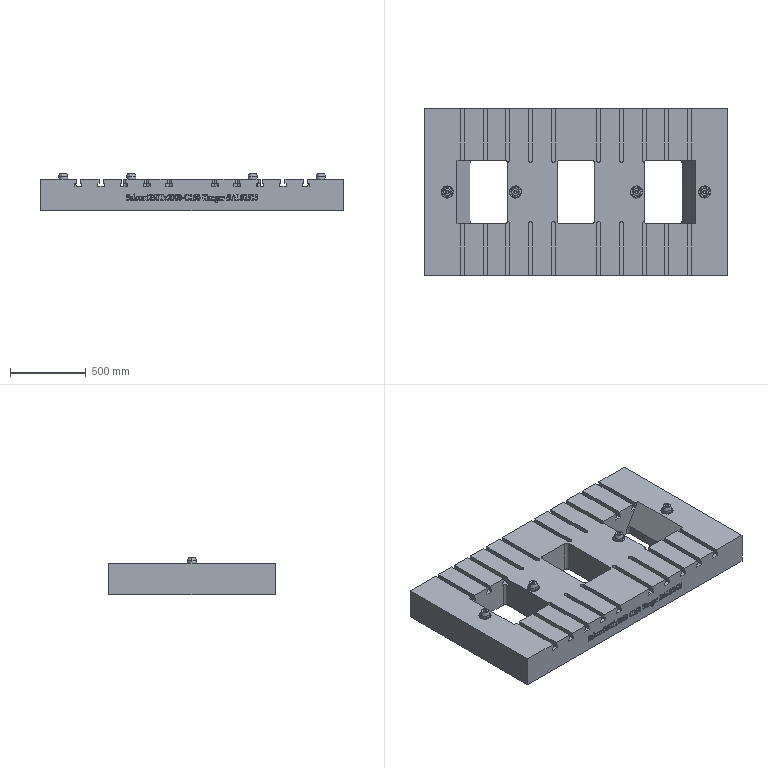Part | CATIA | 5 solids | 982 faces | box 2000 x 1100 x 250 mm | volume 378251028 mm3 | other 426 | plane 407 | cylinder 109 | cone 40 | commonest cylinder face diameters 28 x24 46 x24 21 x16 80 x16 40 x12 18 x8